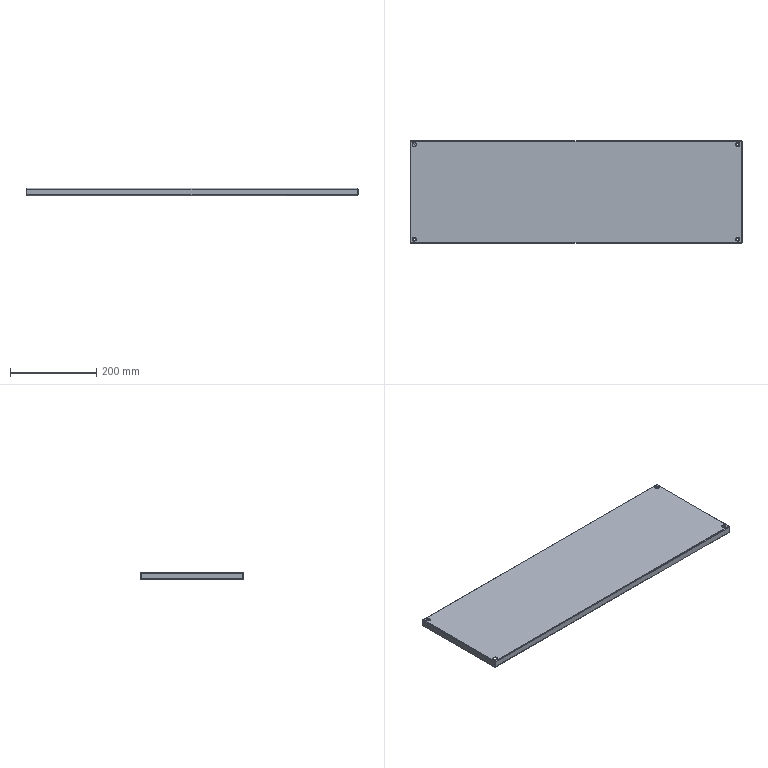Part | SolidWorks | features EdgeFlange 2, Cut 1, FlatPattern 1, HoleWzd 1, SMBaseFlange 1, SheetMetal 1 | 1 solid | 96 faces | box 768 x 238 x 17.5 mm | volume 357698 mm3 | plane 44 | cylinder 36 | spline 16 | commonest cylinder face diameters 5.8 x12 1 x8 4 x8 10 x8